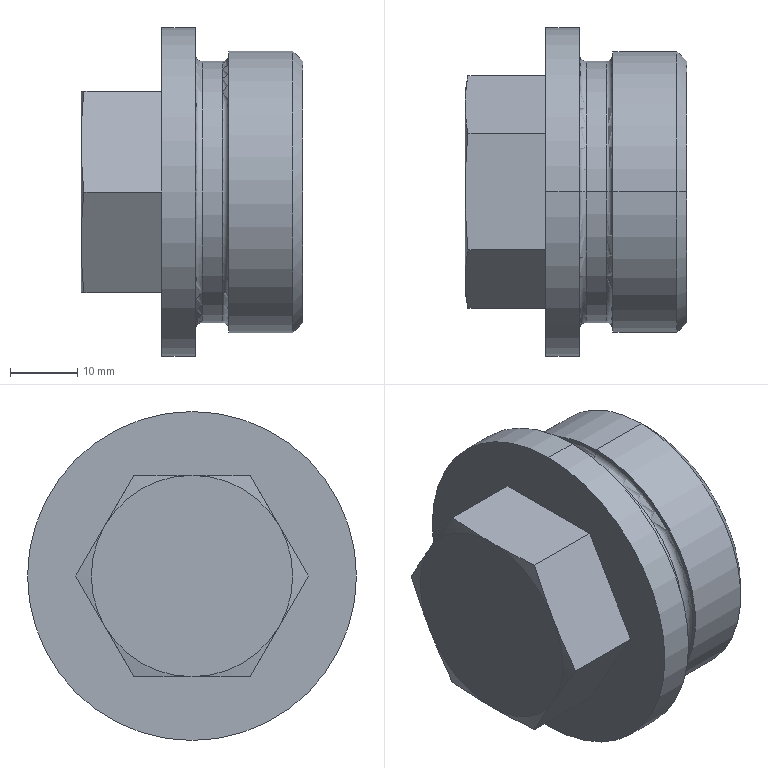Part | SolidWorks | features Boss 1, Cut 1, Fillet 1, Revolution 1 | 1 solid | 29 faces | box 33 x 49 x 49 mm | volume 39818 mm3 | plane 11 | cone 8 | cylinder 6 | torus 4 | commonest cylinder face diameters 38.952 x2 41.91 x2 49 x2
STEP:
#1=CARTESIAN_POINT('',(17.,0.,-20.476));
#2=VERTEX_POINT('',#1);
#3=CARTESIAN_POINT('',(17.,0.,20.476));
#4=VERTEX_POINT('',#3);
#5=CARTESIAN_POINT('',(17.,0.,0.));
#6=DIRECTION('',(-1.,0.,0.));
#7=DIRECTION('',(0.,0.,1.));
#8=AXIS2_PLACEMENT_3D('',#5,#6,#7);
#9=CIRCLE('',#8,20.476);
#10=EDGE_CURVE('',#2,#4,#9,.T.);
#11=ORIENTED_EDGE('',*,*,#10,.F.);
#12=CARTESIAN_POINT('',(18.,0.,-19.476));
#13=VERTEX_POINT('',#12);
#14=CARTESIAN_POINT('',(18.,0.,-20.476));
#15=DIRECTION('',(0.,1.,0.));
#16=DIRECTION('',(0.,0.,1.));
#17=AXIS2_PLACEMENT_3D('',#14,#15,#16);
#18=CIRCLE('',#17,1.);
#19=EDGE_CURVE('',#2,#13,#18,.T.);
#20=ORIENTED_EDGE('',*,*,#19,.T.);
#21=CARTESIAN_POINT('',(18.,0.,19.476));
#22=VERTEX_POINT('',#21);
#23=CARTESIAN_POINT('',(18.,0.,0.));
#24=DIRECTION('',(1.,0.,0.));
#25=DIRECTION('',(0.,0.,1.));
#26=AXIS2_PLACEMENT_3D('',#23,#24,#25);
#27=CIRCLE('',#26,19.476);
#28=EDGE_CURVE('',#22,#13,#27,.T.);
#29=ORIENTED_EDGE('',*,*,#28,.F.);
#30=CARTESIAN_POINT('',(18.,0.,20.476));
#31=DIRECTION('',(0.,-1.,0.));
#32=DIRECTION('',(0.,0.,-1.));
#33=AXIS2_PLACEMENT_3D('',#30,#31,#32);
#34=CIRCLE('',#33,1.);
#35=EDGE_CURVE('',#4,#22,#34,.T.);
#36=ORIENTED_EDGE('',*,*,#35,.F.);
#37=EDGE_LOOP('',(#11,#20,#29,#36));
#38=FACE_OUTER_BOUND('',#37,.T.);
#39=CARTESIAN_POINT('',(18.,0.,0.));
#40=DIRECTION('',(-1.,0.,0.));
#41=DIRECTION('',(0.,0.,1.));
#42=AXIS2_PLACEMENT_3D('',#39,#40,#41);
#43=TOROIDAL_SURFACE('',#42,20.476,1.);
#44=ADVANCED_FACE('',(#38),#43,.F.);
#45=CARTESIAN_POINT('',(22.,0.,20.476));
#46=VERTEX_POINT('',#45);
#47=CARTESIAN_POINT('',(22.,0.,-20.476));
#48=VERTEX_POINT('',#47);
#49=CARTESIAN_POINT('',(22.,0.,0.));
#50=DIRECTION('',(1.,0.,0.));
#51=DIRECTION('',(0.,0.,-1.));
#52=AXIS2_PLACEMENT_3D('',#49,#50,#51);
#53=CIRCLE('',#52,20.476);
#54=EDGE_CURVE('',#46,#48,#53,.T.);
#55=ORIENTED_EDGE('',*,*,#54,.F.);
#56=CARTESIAN_POINT('',(21.,0.,19.476));
#57=VERTEX_POINT('',#56);
#58=CARTESIAN_POINT('',(21.,0.,20.476));
#59=DIRECTION('',(0.,1.,0.));
#60=DIRECTION('',(0.,0.,1.));
#61=AXIS2_PLACEMENT_3D('',#58,#59,#60);
#62=CIRCLE('',#61,1.);
#63=EDGE_CURVE('',#46,#57,#62,.T.);
#64=ORIENTED_EDGE('',*,*,#63,.T.);
#65=CARTESIAN_POINT('',(21.,0.,-19.476));
#66=VERTEX_POINT('',#65);
#67=CARTESIAN_POINT('',(21.,0.,0.));
#68=DIRECTION('',(-1.,0.,0.));
#69=DIRECTION('',(0.,0.,-1.));
#70=AXIS2_PLACEMENT_3D('',#67,#68,#69);
#71=CIRCLE('',#70,19.476);
#72=EDGE_CURVE('',#66,#57,#71,.T.);
#73=ORIENTED_EDGE('',*,*,#72,.F.);
#74=CARTESIAN_POINT('',(21.,0.,-20.476));
#75=DIRECTION('',(0.,-1.,0.));
#76=DIRECTION('',(0.,0.,-1.));
#77=AXIS2_PLACEMENT_3D('',#74,#75,#76);
#78=CIRCLE('',#77,1.);
#79=EDGE_CURVE('',#48,#66,#78,.T.);
#80=ORIENTED_EDGE('',*,*,#79,.F.);
#81=EDGE_LOOP('',(#55,#64,#73,#80));
#82=FACE_OUTER_BOUND('',#81,.T.);
#83=CARTESIAN_POINT('',(21.,0.,0.));
#84=DIRECTION('',(1.,0.,0.));
#85=DIRECTION('',(0.,0.,-1.));
#86=AXIS2_PLACEMENT_3D('',#83,#84,#85);
#87=TOROIDAL_SURFACE('',#86,20.476,1.);
#88=ADVANCED_FACE('',(#82),#87,.F.);
#89=CARTESIAN_POINT('',(33.,0.,19.476));
#90=VERTEX_POINT('',#89);
#91=CARTESIAN_POINT('',(33.,0.,-19.476));
#92=VERTEX_POINT('',#91);
#93=CARTESIAN_POINT('',(33.,0.,0.));
#94=DIRECTION('',(-1.,0.,0.));
#95=DIRECTION('',(0.,0.,1.));
#96=AXIS2_PLACEMENT_3D('',#93,#94,#95);
#97=CIRCLE('',#96,19.476);
#98=EDGE_CURVE('',#90,#92,#97,.T.);
#99=ORIENTED_EDGE('',*,*,#98,.T.);
#100=CARTESIAN_POINT('',(31.521,0.,-20.955));
#101=VERTEX_POINT('',#100);
#102=CARTESIAN_POINT('',(33.,0.,-19.476));
#103=DIRECTION('',(-0.7071,0.,-0.7071));
#104=VECTOR('',#103,1000.);
#105=LINE('',#102,#104);
#106=EDGE_CURVE('',#92,#101,#105,.T.);
#107=ORIENTED_EDGE('',*,*,#106,.T.);
#108=CARTESIAN_POINT('',(31.521,0.,20.955));
#109=VERTEX_POINT('',#108);
#110=CARTESIAN_POINT('',(31.521,0.,0.));
#111=DIRECTION('',(-1.,0.,0.));
#112=DIRECTION('',(0.,0.,1.));
#113=AXIS2_PLACEMENT_3D('',#110,#111,#112);
#114=CIRCLE('',#113,20.955);
#115=EDGE_CURVE('',#109,#101,#114,.T.);
#116=ORIENTED_EDGE('',*,*,#115,.F.);
#117=CARTESIAN_POINT('',(33.,0.,19.476));
#118=DIRECTION('',(-0.7071,0.,0.7071));
#119=VECTOR('',#118,1000.);
#120=LINE('',#117,#119);
#121=EDGE_CURVE('',#90,#109,#120,.T.);
#122=ORIENTED_EDGE('',*,*,#121,.F.);
#123=EDGE_LOOP('',(#99,#107,#116,#122));
#124=FACE_OUTER_BOUND('',#123,.T.);
#125=CARTESIAN_POINT('',(33.,0.,0.));
#126=DIRECTION('',(-1.,0.,0.));
#127=DIRECTION('',(0.,0.,1.));
#128=AXIS2_PLACEMENT_3D('',#125,#126,#127);
#129=CONICAL_SURFACE('',#128,19.476,0.7854);
#130=ADVANCED_FACE('',(#124),#129,.T.);
#131=ORIENTED_EDGE('',*,*,#115,.T.);
#132=CARTESIAN_POINT('',(22.,0.,-20.955));
#133=VERTEX_POINT('',#132);
#134=CARTESIAN_POINT('',(0.,0.,-20.955));
#135=DIRECTION('',(-1.,0.,0.));
#136=VECTOR('',#135,1000.);
#137=LINE('',#134,#136);
#138=EDGE_CURVE('',#101,#133,#137,.T.);
#139=ORIENTED_EDGE('',*,*,#138,.T.);
#140=CARTESIAN_POINT('',(22.,0.,20.955));
#141=VERTEX_POINT('',#140);
#142=CARTESIAN_POINT('',(22.,0.,0.));
#143=DIRECTION('',(-1.,0.,0.));
#144=DIRECTION('',(0.,0.,1.));
#145=AXIS2_PLACEMENT_3D('',#142,#143,#144);
#146=CIRCLE('',#145,20.955);
#147=EDGE_CURVE('',#141,#133,#146,.T.);
#148=ORIENTED_EDGE('',*,*,#147,.F.);
#149=CARTESIAN_POINT('',(0.,0.,20.955));
#150=DIRECTION('',(-1.,0.,0.));
#151=VECTOR('',#150,1000.);
#152=LINE('',#149,#151);
#153=EDGE_CURVE('',#109,#141,#152,.T.);
#154=ORIENTED_EDGE('',*,*,#153,.F.);
#155=EDGE_LOOP('',(#131,#139,#148,#154));
#156=FACE_OUTER_BOUND('',#155,.T.);
#157=CARTESIAN_POINT('',(0.,0.,0.));
#158=DIRECTION('',(-1.,0.,0.));
#159=DIRECTION('',(0.,0.,1.));
#160=AXIS2_PLACEMENT_3D('',#157,#158,#159);
#161=CYLINDRICAL_SURFACE('',#160,20.955);
#162=ADVANCED_FACE('',(#156),#161,.T.);
#163=CARTESIAN_POINT('',(21.,0.,0.));
#164=DIRECTION('',(-1.,0.,0.));
#165=DIRECTION('',(0.,0.,-1.));
#166=AXIS2_PLACEMENT_3D('',#163,#164,#165);
#167=CIRCLE('',#166,19.476);
#168=EDGE_CURVE('',#57,#66,#167,.T.);
#169=ORIENTED_EDGE('',*,*,#168,.T.);
#170=CARTESIAN_POINT('',(0.,0.,-19.476));
#171=DIRECTION('',(-1.,0.,0.));
#172=VECTOR('',#171,1000.);
#173=LINE('',#170,#172);
#174=EDGE_CURVE('',#66,#13,#173,.T.);
#175=ORIENTED_EDGE('',*,*,#174,.T.);
#176=CARTESIAN_POINT('',(18.,0.,0.));
#177=DIRECTION('',(1.,0.,0.));
#178=DIRECTION('',(0.,0.,1.));
#179=AXIS2_PLACEMENT_3D('',#176,#177,#178);
#180=CIRCLE('',#179,19.476);
#181=EDGE_CURVE('',#13,#22,#180,.T.);
#182=ORIENTED_EDGE('',*,*,#181,.T.);
#183=CARTESIAN_POINT('',(0.,0.,19.476));
#184=DIRECTION('',(-1.,0.,0.));
#185=VECTOR('',#184,1000.);
#186=LINE('',#183,#185);
#187=EDGE_CURVE('',#57,#22,#186,.T.);
#188=ORIENTED_EDGE('',*,*,#187,.F.);
#189=EDGE_LOOP('',(#169,#175,#182,#188));
#190=FACE_OUTER_BOUND('',#189,.T.);
#191=CARTESIAN_POINT('',(0.,0.,0.));
#192=DIRECTION('',(-1.,0.,0.));
#193=DIRECTION('',(0.,0.,1.));
#194=AXIS2_PLACEMENT_3D('',#191,#192,#193);
#195=CYLINDRICAL_SURFACE('',#194,19.476);
#196=ADVANCED_FACE('',(#190),#195,.T.);
#197=CARTESIAN_POINT('',(17.,0.,24.5));
#198=VERTEX_POINT('',#197);
#199=CARTESIAN_POINT('',(17.,0.,-24.5));
#200=VERTEX_POINT('',#199);
#201=CARTESIAN_POINT('',(17.,0.,0.));
#202=DIRECTION('',(-1.,0.,0.));
#203=DIRECTION('',(0.,0.,1.));
#204=AXIS2_PLACEMENT_3D('',#201,#202,#203);
#205=CIRCLE('',#204,24.5);
#206=EDGE_CURVE('',#198,#200,#205,.T.);
#207=ORIENTED_EDGE('',*,*,#206,.T.);
#208=CARTESIAN_POINT('',(12.,0.,-24.5));
#209=VERTEX_POINT('',#208);
#210=CARTESIAN_POINT('',(0.,0.,-24.5));
#211=DIRECTION('',(-1.,0.,0.));
#212=VECTOR('',#211,1000.);
#213=LINE('',#210,#212);
#214=EDGE_CURVE('',#200,#209,#213,.T.);
#215=ORIENTED_EDGE('',*,*,#214,.T.);
#216=CARTESIAN_POINT('',(12.,0.,24.5));
#217=VERTEX_POINT('',#216);
#218=CARTESIAN_POINT('',(12.,0.,0.));
#219=DIRECTION('',(-1.,0.,0.));
#220=DIRECTION('',(0.,0.,1.));
#221=AXIS2_PLACEMENT_3D('',#218,#219,#220);
#222=CIRCLE('',#221,24.5);
#223=EDGE_CURVE('',#217,#209,#222,.T.);
#224=ORIENTED_EDGE('',*,*,#223,.F.);
#225=CARTESIAN_POINT('',(0.,0.,24.5));
#226=DIRECTION('',(-1.,0.,0.));
#227=VECTOR('',#226,1000.);
#228=LINE('',#225,#227);
#229=EDGE_CURVE('',#198,#217,#228,.T.);
#230=ORIENTED_EDGE('',*,*,#229,.F.);
#231=EDGE_LOOP('',(#207,#215,#224,#230));
#232=FACE_OUTER_BOUND('',#231,.T.);
#233=CARTESIAN_POINT('',(0.,0.,0.));
#234=DIRECTION('',(-1.,0.,0.));
#235=DIRECTION('',(0.,0.,1.));
#236=AXIS2_PLACEMENT_3D('',#233,#234,#235);
#237=CYLINDRICAL_SURFACE('',#236,24.5);
#238=ADVANCED_FACE('',(#232),#237,.T.);
#239=CARTESIAN_POINT('',(12.,8.66,-15.));
#240=VERTEX_POINT('',#239);
#241=CARTESIAN_POINT('',(0.4092,8.66,-15.));
#242=VERTEX_POINT('',#241);
#243=CARTESIAN_POINT('',(57.826,8.66,-15.));
#244=DIRECTION('',(-1.,0.,0.));
#245=VECTOR('',#244,1000.);
#246=LINE('',#243,#245);
#247=EDGE_CURVE('',#240,#242,#246,.T.);
#248=ORIENTED_EDGE('',*,*,#247,.T.);
#249=CARTESIAN_POINT('',(0.,12.99,-7.5));
#250=VERTEX_POINT('',#249);
#251=CARTESIAN_POINT('',(0.4092,8.66,-15.));
#252=CARTESIAN_POINT('',(0.2819,9.382,-13.75));
#253=CARTESIAN_POINT('',(0.1786,10.104,-12.5));
#254=CARTESIAN_POINT('',(0.03741,11.547,-10.));
#255=CARTESIAN_POINT('',(0.,12.269,-8.75));
#256=CARTESIAN_POINT('',(0.,12.99,-7.5));
#257=B_SPLINE_CURVE_WITH_KNOTS('',3,(#251,#252,#253,#254,#255,#256),.UNSPECIFIED.,.F.,.F.,(4,2,4),(0.000000231,0.00433,0.00866),.UNSPECIFIED.);
#258=EDGE_CURVE('',#242,#250,#257,.T.);
#259=ORIENTED_EDGE('',*,*,#258,.T.);
#260=CARTESIAN_POINT('',(0.4092,17.321,0.));
#261=VERTEX_POINT('',#260);
#262=CARTESIAN_POINT('',(0.,12.99,-7.5));
#263=CARTESIAN_POINT('',(0.,13.712,-6.25));
#264=CARTESIAN_POINT('',(0.03741,14.434,-5.));
#265=CARTESIAN_POINT('',(0.1786,15.877,-2.5));
#266=CARTESIAN_POINT('',(0.2819,16.599,-1.25));
#267=CARTESIAN_POINT('',(0.4092,17.321,0.));
#268=B_SPLINE_CURVE_WITH_KNOTS('',3,(#262,#263,#264,#265,#266,#267),.UNSPECIFIED.,.F.,.F.,(4,2,4),(0.00866,0.01299,0.01732),.UNSPECIFIED.);
#269=EDGE_CURVE('',#250,#261,#268,.T.);
#270=ORIENTED_EDGE('',*,*,#269,.T.);
#271=CARTESIAN_POINT('',(12.,17.321,0.));
#272=VERTEX_POINT('',#271);
#273=CARTESIAN_POINT('',(57.826,17.321,0.));
#274=DIRECTION('',(-1.,0.,0.));
#275=VECTOR('',#274,1000.);
#276=LINE('',#273,#275);
#277=EDGE_CURVE('',#272,#261,#276,.T.);
#278=ORIENTED_EDGE('',*,*,#277,.F.);
#279=CARTESIAN_POINT('',(12.,17.321,0.));
#280=DIRECTION('',(0.,-0.5,-0.866));
#281=VECTOR('',#280,1000.);
#282=LINE('',#279,#281);
#283=EDGE_CURVE('',#272,#240,#282,.T.);
#284=ORIENTED_EDGE('',*,*,#283,.T.);
#285=EDGE_LOOP('',(#248,#259,#270,#278,#284));
#286=FACE_OUTER_BOUND('',#285,.T.);
#287=CARTESIAN_POINT('',(57.826,17.321,0.));
#288=DIRECTION('',(0.,0.866,-0.5));
#289=DIRECTION('',(0.,0.5,0.866));
#290=AXIS2_PLACEMENT_3D('',#287,#288,#289);
#291=PLANE('',#290);
#292=ADVANCED_FACE('',(#286),#291,.T.);
#293=CARTESIAN_POINT('',(12.,-8.66,-15.));
#294=VERTEX_POINT('',#293);
#295=CARTESIAN_POINT('',(0.4092,-8.66,-15.));
#296=VERTEX_POINT('',#295);
#297=CARTESIAN_POINT('',(57.826,-8.66,-15.));
#298=DIRECTION('',(-1.,0.,0.));
#299=VECTOR('',#298,1000.);
#300=LINE('',#297,#299);
#301=EDGE_CURVE('',#294,#296,#300,.T.);
#302=ORIENTED_EDGE('',*,*,#301,.T.);
#303=CARTESIAN_POINT('',(0.,0.,-15.));
#304=VERTEX_POINT('',#303);
#305=CARTESIAN_POINT('',(0.4092,-8.66,-15.));
#306=CARTESIAN_POINT('',(0.2821,-7.219,-15.));
#307=CARTESIAN_POINT('',(0.1786,-5.773,-15.));
#308=CARTESIAN_POINT('',(0.03738,-2.886,-15.));
#309=CARTESIAN_POINT('',(0.,-1.443,-15.));
#310=CARTESIAN_POINT('',(0.,0.,-15.));
#311=B_SPLINE_CURVE_WITH_KNOTS('',3,(#305,#306,#307,#308,#309,#310),.UNSPECIFIED.,.F.,.F.,(4,2,4),(0.01454,0.01888,0.02322),.UNSPECIFIED.);
#312=EDGE_CURVE('',#296,#304,#311,.T.);
#313=ORIENTED_EDGE('',*,*,#312,.T.);
#314=CARTESIAN_POINT('',(0.,0.,-15.));
#315=CARTESIAN_POINT('',(0.,1.445,-15.));
#316=CARTESIAN_POINT('',(0.03747,2.888,-15.));
#317=CARTESIAN_POINT('',(0.1787,5.775,-15.));
#318=CARTESIAN_POINT('',(0.282,7.218,-15.));
#319=CARTESIAN_POINT('',(0.4092,8.66,-15.));
#320=B_SPLINE_CURVE_WITH_KNOTS('',3,(#314,#315,#316,#317,#318,#319),.UNSPECIFIED.,.F.,.F.,(4,2,4),(0.02322,0.02756,0.03191),.UNSPECIFIED.);
#321=EDGE_CURVE('',#304,#242,#320,.T.);
#322=ORIENTED_EDGE('',*,*,#321,.T.);
#323=ORIENTED_EDGE('',*,*,#247,.F.);
#324=CARTESIAN_POINT('',(12.,8.66,-15.));
#325=DIRECTION('',(0.,-1.,0.));
#326=VECTOR('',#325,1000.);
#327=LINE('',#324,#326);
#328=EDGE_CURVE('',#240,#294,#327,.T.);
#329=ORIENTED_EDGE('',*,*,#328,.T.);
#330=EDGE_LOOP('',(#302,#313,#322,#323,#329));
#331=FACE_OUTER_BOUND('',#330,.T.);
#332=CARTESIAN_POINT('',(57.826,8.66,-15.));
#333=DIRECTION('',(0.,0.,-1.));
#334=DIRECTION('',(0.,1.,0.));
#335=AXIS2_PLACEMENT_3D('',#332,#333,#334);
#336=PLANE('',#335);
#337=ADVANCED_FACE('',(#331),#336,.T.);
#338=CARTESIAN_POINT('',(12.,-17.321,0.));
#339=VERTEX_POINT('',#338);
#340=CARTESIAN_POINT('',(0.4092,-17.321,0.));
#341=VERTEX_POINT('',#340);
#342=CARTESIAN_POINT('',(57.826,-17.321,0.));
#343=DIRECTION('',(-1.,0.,0.));
#344=VECTOR('',#343,1000.);
#345=LINE('',#342,#344);
#346=EDGE_CURVE('',#339,#341,#345,.T.);
#347=ORIENTED_EDGE('',*,*,#346,.T.);
#348=CARTESIAN_POINT('',(0.,-12.99,-7.5));
#349=VERTEX_POINT('',#348);
#350=CARTESIAN_POINT('',(0.4092,-17.321,0.));
#351=CARTESIAN_POINT('',(0.2819,-16.599,-1.25));
#352=CARTESIAN_POINT('',(0.1786,-15.877,-2.5));
#353=CARTESIAN_POINT('',(0.03741,-14.434,-5.));
#354=CARTESIAN_POINT('',(0.,-13.712,-6.25));
#355=CARTESIAN_POINT('',(0.,-12.99,-7.5));
#356=B_SPLINE_CURVE_WITH_KNOTS('',3,(#350,#351,#352,#353,#354,#355),.UNSPECIFIED.,.F.,.F.,(4,2,4),(0.000000231,0.00433,0.00866),.UNSPECIFIED.);
#357=EDGE_CURVE('',#341,#349,#356,.T.);
#358=ORIENTED_EDGE('',*,*,#357,.T.);
#359=CARTESIAN_POINT('',(0.,-12.99,-7.5));
#360=CARTESIAN_POINT('',(0.,-12.269,-8.75));
#361=CARTESIAN_POINT('',(0.03741,-11.547,-10.));
#362=CARTESIAN_POINT('',(0.1786,-10.104,-12.5));
#363=CARTESIAN_POINT('',(0.2819,-9.382,-13.75));
#364=CARTESIAN_POINT('',(0.4092,-8.66,-15.));
#365=B_SPLINE_CURVE_WITH_KNOTS('',3,(#359,#360,#361,#362,#363,#364),.UNSPECIFIED.,.F.,.F.,(4,2,4),(0.00866,0.01299,0.01732),.UNSPECIFIED.);
#366=EDGE_CURVE('',#349,#296,#365,.T.);
#367=ORIENTED_EDGE('',*,*,#366,.T.);
#368=ORIENTED_EDGE('',*,*,#301,.F.);
#369=CARTESIAN_POINT('',(12.,-8.66,-15.));
#370=DIRECTION('',(0.,-0.5,0.866));
#371=VECTOR('',#370,1000.);
#372=LINE('',#369,#371);
#373=EDGE_CURVE('',#294,#339,#372,.T.);
#374=ORIENTED_EDGE('',*,*,#373,.T.);
#375=EDGE_LOOP('',(#347,#358,#367,#368,#374));
#376=FACE_OUTER_BOUND('',#375,.T.);
#377=CARTESIAN_POINT('',(57.826,-8.66,-15.));
#378=DIRECTION('',(0.,-0.866,-0.5));
#379=DIRECTION('',(0.,0.5,-0.866));
#380=AXIS2_PLACEMENT_3D('',#377,#378,#379);
#381=PLANE('',#380);
#382=ADVANCED_FACE('',(#376),#381,.T.);
#383=CARTESIAN_POINT('',(12.,-8.66,15.));
#384=VERTEX_POINT('',#383);
#385=CARTESIAN_POINT('',(0.4092,-8.66,15.));
#386=VERTEX_POINT('',#385);
#387=CARTESIAN_POINT('',(57.826,-8.66,15.));
#388=DIRECTION('',(-1.,0.,0.));
#389=VECTOR('',#388,1000.);
#390=LINE('',#387,#389);
#391=EDGE_CURVE('',#384,#386,#390,.T.);
#392=ORIENTED_EDGE('',*,*,#391,.T.);
#393=CARTESIAN_POINT('',(0.,-12.99,7.5));
#394=VERTEX_POINT('',#393);
#395=CARTESIAN_POINT('',(0.4092,-8.66,15.));
#396=CARTESIAN_POINT('',(0.2819,-9.382,13.75));
#397=CARTESIAN_POINT('',(0.1786,-10.104,12.5));
#398=CARTESIAN_POINT('',(0.03741,-11.547,10.));
#399=CARTESIAN_POINT('',(0.,-12.269,8.75));
#400=CARTESIAN_POINT('',(0.,-12.99,7.5));
#401=B_SPLINE_CURVE_WITH_KNOTS('',3,(#395,#396,#397,#398,#399,#400),.UNSPECIFIED.,.F.,.F.,(4,2,4),(0.000000231,0.00433,0.00866),.UNSPECIFIED.);
#402=EDGE_CURVE('',#386,#394,#401,.T.);
#403=ORIENTED_EDGE('',*,*,#402,.T.);
#404=CARTESIAN_POINT('',(0.,-12.99,7.5));
#405=CARTESIAN_POINT('',(0.,-13.712,6.25));
#406=CARTESIAN_POINT('',(0.03741,-14.434,5.));
#407=CARTESIAN_POINT('',(0.1786,-15.877,2.5));
#408=CARTESIAN_POINT('',(0.2819,-16.599,1.25));
#409=CARTESIAN_POINT('',(0.4092,-17.321,0.));
#410=B_SPLINE_CURVE_WITH_KNOTS('',3,(#404,#405,#406,#407,#408,#409),.UNSPECIFIED.,.F.,.F.,(4,2,4),(0.00866,0.01299,0.01732),.UNSPECIFIED.);
#411=EDGE_CURVE('',#394,#341,#410,.T.);
#412=ORIENTED_EDGE('',*,*,#411,.T.);
#413=ORIENTED_EDGE('',*,*,#346,.F.);
#414=CARTESIAN_POINT('',(12.,-17.321,0.));
#415=DIRECTION('',(0.,0.5,0.866));
#416=VECTOR('',#415,1000.);
#417=LINE('',#414,#416);
#418=EDGE_CURVE('',#339,#384,#417,.T.);
#419=ORIENTED_EDGE('',*,*,#418,.T.);
#420=EDGE_LOOP('',(#392,#403,#412,#413,#419));
#421=FACE_OUTER_BOUND('',#420,.T.);
#422=CARTESIAN_POINT('',(57.826,-17.321,0.));
#423=DIRECTION('',(0.,-0.866,0.5));
#424=DIRECTION('',(0.,-0.5,-0.866));
#425=AXIS2_PLACEMENT_3D('',#422,#423,#424);
#426=PLANE('',#425);
#427=ADVANCED_FACE('',(#421),#426,.T.);
#428=CARTESIAN_POINT('',(12.,8.66,15.));
#429=VERTEX_POINT('',#428);
#430=CARTESIAN_POINT('',(0.4092,8.66,15.));
#431=VERTEX_POINT('',#430);
#432=CARTESIAN_POINT('',(57.826,8.66,15.));
#433=DIRECTION('',(-1.,0.,0.));
#434=VECTOR('',#433,1000.);
#435=LINE('',#432,#434);
#436=EDGE_CURVE('',#429,#431,#435,.T.);
#437=ORIENTED_EDGE('',*,*,#436,.T.);
#438=CARTESIAN_POINT('',(0.,0.,15.));
#439=VERTEX_POINT('',#438);
#440=CARTESIAN_POINT('',(0.4092,8.66,15.));
#441=CARTESIAN_POINT('',(0.282,7.218,15.));
#442=CARTESIAN_POINT('',(0.1787,5.775,15.));
#443=CARTESIAN_POINT('',(0.03747,2.888,15.));
#444=CARTESIAN_POINT('',(0.,1.445,15.));
#445=CARTESIAN_POINT('',(0.,0.,15.));
#446=B_SPLINE_CURVE_WITH_KNOTS('',3,(#440,#441,#442,#443,#444,#445),.UNSPECIFIED.,.F.,.F.,(4,2,4),(0.0406,0.04494,0.04928),.UNSPECIFIED.);
#447=EDGE_CURVE('',#431,#439,#446,.T.);
#448=ORIENTED_EDGE('',*,*,#447,.T.);
#449=CARTESIAN_POINT('',(0.,0.,15.));
#450=CARTESIAN_POINT('',(0.,-1.443,15.));
#451=CARTESIAN_POINT('',(0.03738,-2.886,15.));
#452=CARTESIAN_POINT('',(0.1786,-5.773,15.));
#453=CARTESIAN_POINT('',(0.2821,-7.219,15.));
#454=CARTESIAN_POINT('',(0.4092,-8.66,15.));
#455=B_SPLINE_CURVE_WITH_KNOTS('',3,(#449,#450,#451,#452,#453,#454),.UNSPECIFIED.,.F.,.F.,(4,2,4),(0.04928,0.05362,0.05795),.UNSPECIFIED.);
#456=EDGE_CURVE('',#439,#386,#455,.T.);
#457=ORIENTED_EDGE('',*,*,#456,.T.);
#458=ORIENTED_EDGE('',*,*,#391,.F.);
#459=CARTESIAN_POINT('',(12.,-8.66,15.));
#460=DIRECTION('',(0.,1.,0.));
#461=VECTOR('',#460,1000.);
#462=LINE('',#459,#461);
#463=EDGE_CURVE('',#384,#429,#462,.T.);
#464=ORIENTED_EDGE('',*,*,#463,.T.);
#465=EDGE_LOOP('',(#437,#448,#457,#458,#464));
#466=FACE_OUTER_BOUND('',#465,.T.);
#467=CARTESIAN_POINT('',(57.826,-8.66,15.));
#468=DIRECTION('',(0.,0.,1.));
#469=DIRECTION('',(0.,-1.,0.));
#470=AXIS2_PLACEMENT_3D('',#467,#468,#469);
#471=PLANE('',#470);
#472=ADVANCED_FACE('',(#466),#471,.T.);
#473=ORIENTED_EDGE('',*,*,#277,.T.);
#474=CARTESIAN_POINT('',(0.,12.99,7.5));
#475=VERTEX_POINT('',#474);
#476=CARTESIAN_POINT('',(0.4092,17.321,0.));
#477=CARTESIAN_POINT('',(0.2819,16.599,1.25));
#478=CARTESIAN_POINT('',(0.1786,15.877,2.5));
#479=CARTESIAN_POINT('',(0.03741,14.434,5.));
#480=CARTESIAN_POINT('',(0.,13.712,6.25));
#481=CARTESIAN_POINT('',(0.,12.99,7.5));
#482=B_SPLINE_CURVE_WITH_KNOTS('',3,(#476,#477,#478,#479,#480,#481),.UNSPECIFIED.,.F.,.F.,(4,2,4),(0.000000231,0.00433,0.00866),.UNSPECIFIED.);
#483=EDGE_CURVE('',#261,#475,#482,.T.);
#484=ORIENTED_EDGE('',*,*,#483,.T.);
#485=CARTESIAN_POINT('',(0.,12.99,7.5));
#486=CARTESIAN_POINT('',(0.,12.269,8.75));
#487=CARTESIAN_POINT('',(0.03741,11.547,10.));
#488=CARTESIAN_POINT('',(0.1786,10.104,12.5));
#489=CARTESIAN_POINT('',(0.2819,9.382,13.75));
#490=CARTESIAN_POINT('',(0.4092,8.66,15.));
#491=B_SPLINE_CURVE_WITH_KNOTS('',3,(#485,#486,#487,#488,#489,#490),.UNSPECIFIED.,.F.,.F.,(4,2,4),(0.00866,0.01299,0.01732),.UNSPECIFIED.);
#492=EDGE_CURVE('',#475,#431,#491,.T.);
#493=ORIENTED_EDGE('',*,*,#492,.T.);
#494=ORIENTED_EDGE('',*,*,#436,.F.);
#495=CARTESIAN_POINT('',(12.,8.66,15.));
#496=DIRECTION('',(0.,0.5,-0.866));
#497=VECTOR('',#496,1000.);
#498=LINE('',#495,#497);
#499=EDGE_CURVE('',#429,#272,#498,.T.);
#500=ORIENTED_EDGE('',*,*,#499,.T.);
#501=EDGE_LOOP('',(#473,#484,#493,#494,#500));
#502=FACE_OUTER_BOUND('',#501,.T.);
#503=CARTESIAN_POINT('',(57.826,8.66,15.));
#504=DIRECTION('',(0.,0.866,0.5));
#505=DIRECTION('',(0.,-0.5,0.866));
#506=AXIS2_PLACEMENT_3D('',#503,#504,#505);
#507=PLANE('',#506);
#508=ADVANCED_FACE('',(#502),#507,.T.);
#509=ORIENTED_EDGE('',*,*,#328,.F.);
#510=ORIENTED_EDGE('',*,*,#283,.F.);
#511=ORIENTED_EDGE('',*,*,#499,.F.);
#512=ORIENTED_EDGE('',*,*,#463,.F.);
#513=ORIENTED_EDGE('',*,*,#418,.F.);
#514=ORIENTED_EDGE('',*,*,#373,.F.);
#515=EDGE_LOOP('',(#509,#510,#511,#512,#513,#514));
#516=FACE_BOUND('',#515,.T.);
#517=ORIENTED_EDGE('',*,*,#223,.T.);
#518=CARTESIAN_POINT('',(12.,0.,0.));
#519=DIRECTION('',(-1.,0.,0.));
#520=DIRECTION('',(0.,0.,1.));
#521=AXIS2_PLACEMENT_3D('',#518,#519,#520);
#522=CIRCLE('',#521,24.5);
#523=EDGE_CURVE('',#209,#217,#522,.T.);
#524=ORIENTED_EDGE('',*,*,#523,.T.);
#525=EDGE_LOOP('',(#517,#524));
#526=FACE_OUTER_BOUND('',#525,.T.);
#527=CARTESIAN_POINT('',(12.,24.5,0.));
#528=DIRECTION('',(1.,0.,0.));
#529=DIRECTION('',(0.,0.,-1.));
#530=AXIS2_PLACEMENT_3D('',#527,#528,#529);
#531=PLANE('',#530);
#532=ADVANCED_FACE('',(#516,#526),#531,.F.);
#533=ORIENTED_EDGE('',*,*,#214,.F.);
#534=CARTESIAN_POINT('',(17.,0.,0.));
#535=DIRECTION('',(-1.,0.,0.));
#536=DIRECTION('',(0.,0.,1.));
#537=AXIS2_PLACEMENT_3D('',#534,#535,#536);
#538=CIRCLE('',#537,24.5);
#539=EDGE_CURVE('',#200,#198,#538,.T.);
#540=ORIENTED_EDGE('',*,*,#539,.T.);
#541=ORIENTED_EDGE('',*,*,#229,.T.);
#542=ORIENTED_EDGE('',*,*,#523,.F.);
#543=EDGE_LOOP('',(#533,#540,#541,#542));
#544=FACE_OUTER_BOUND('',#543,.T.);
#545=CARTESIAN_POINT('',(0.,0.,0.));
#546=DIRECTION('',(-1.,0.,0.));
#547=DIRECTION('',(0.,0.,1.));
#548=AXIS2_PLACEMENT_3D('',#545,#546,#547);
#549=CYLINDRICAL_SURFACE('',#548,24.5);
#550=ADVANCED_FACE('',(#544),#549,.T.);
#551=CARTESIAN_POINT('',(17.,0.,0.));
#552=DIRECTION('',(-1.,0.,0.));
#553=DIRECTION('',(0.,0.,1.));
#554=AXIS2_PLACEMENT_3D('',#551,#552,#553);
#555=CIRCLE('',#554,20.476);
#556=EDGE_CURVE('',#4,#2,#555,.T.);
#557=ORIENTED_EDGE('',*,*,#556,.T.);
#558=ORIENTED_EDGE('',*,*,#10,.T.);
#559=EDGE_LOOP('',(#557,#558));
#560=FACE_BOUND('',#559,.T.);
#561=ORIENTED_EDGE('',*,*,#206,.F.);
#562=ORIENTED_EDGE('',*,*,#539,.F.);
#563=EDGE_LOOP('',(#561,#562));
#564=FACE_OUTER_BOUND('',#563,.T.);
#565=CARTESIAN_POINT('',(17.,19.476,0.));
#566=DIRECTION('',(-1.,0.,0.));
#567=DIRECTION('',(0.,0.,1.));
#568=AXIS2_PLACEMENT_3D('',#565,#566,#567);
#569=PLANE('',#568);
#570=ADVANCED_FACE('',(#560,#564),#569,.F.);
#571=ORIENTED_EDGE('',*,*,#174,.F.);
#572=ORIENTED_EDGE('',*,*,#72,.T.);
#573=ORIENTED_EDGE('',*,*,#187,.T.);
#574=ORIENTED_EDGE('',*,*,#28,.T.);
#575=EDGE_LOOP('',(#571,#572,#573,#574));
#576=FACE_OUTER_BOUND('',#575,.T.);
#577=CARTESIAN_POINT('',(0.,0.,0.));
#578=DIRECTION('',(-1.,0.,0.));
#579=DIRECTION('',(0.,0.,1.));
#580=AXIS2_PLACEMENT_3D('',#577,#578,#579);
#581=CYLINDRICAL_SURFACE('',#580,19.476);
#582=ADVANCED_FACE('',(#576),#581,.T.);
#583=CARTESIAN_POINT('',(22.,0.,0.));
#584=DIRECTION('',(1.,0.,0.));
#585=DIRECTION('',(0.,0.,-1.));
#586=AXIS2_PLACEMENT_3D('',#583,#584,#585);
#587=CIRCLE('',#586,20.476);
#588=EDGE_CURVE('',#48,#46,#587,.T.);
#589=ORIENTED_EDGE('',*,*,#588,.T.);
#590=ORIENTED_EDGE('',*,*,#54,.T.);
#591=EDGE_LOOP('',(#589,#590));
#592=FACE_BOUND('',#591,.T.);
#593=ORIENTED_EDGE('',*,*,#147,.T.);
#594=CARTESIAN_POINT('',(22.,0.,0.));
#595=DIRECTION('',(-1.,0.,0.));
#596=DIRECTION('',(0.,0.,1.));
#597=AXIS2_PLACEMENT_3D('',#594,#595,#596);
#598=CIRCLE('',#597,20.955);
#599=EDGE_CURVE('',#133,#141,#598,.T.);
#600=ORIENTED_EDGE('',*,*,#599,.T.);
#601=EDGE_LOOP('',(#593,#600));
#602=FACE_OUTER_BOUND('',#601,.T.);
#603=CARTESIAN_POINT('',(22.,20.955,0.));
#604=DIRECTION('',(1.,0.,0.));
#605=DIRECTION('',(0.,0.,-1.));
#606=AXIS2_PLACEMENT_3D('',#603,#604,#605);
#607=PLANE('',#606);
#608=ADVANCED_FACE('',(#592,#602),#607,.F.);
#609=ORIENTED_EDGE('',*,*,#138,.F.);
#610=CARTESIAN_POINT('',(31.521,0.,0.));
#611=DIRECTION('',(-1.,0.,0.));
#612=DIRECTION('',(0.,0.,1.));
#613=AXIS2_PLACEMENT_3D('',#610,#611,#612);
#614=CIRCLE('',#613,20.955);
#615=EDGE_CURVE('',#101,#109,#614,.T.);
#616=ORIENTED_EDGE('',*,*,#615,.T.);
#617=ORIENTED_EDGE('',*,*,#153,.T.);
#618=ORIENTED_EDGE('',*,*,#599,.F.);
#619=EDGE_LOOP('',(#609,#616,#617,#618));
#620=FACE_OUTER_BOUND('',#619,.T.);
#621=CARTESIAN_POINT('',(0.,0.,0.));
#622=DIRECTION('',(-1.,0.,0.));
#623=DIRECTION('',(0.,0.,1.));
#624=AXIS2_PLACEMENT_3D('',#621,#622,#623);
#625=CYLINDRICAL_SURFACE('',#624,20.955);
#626=ADVANCED_FACE('',(#620),#625,.T.);
#627=ORIENTED_EDGE('',*,*,#106,.F.);
#628=CARTESIAN_POINT('',(33.,0.,0.));
#629=DIRECTION('',(-1.,0.,0.));
#630=DIRECTION('',(0.,0.,1.));
#631=AXIS2_PLACEMENT_3D('',#628,#629,#630);
#632=CIRCLE('',#631,19.476);
#633=EDGE_CURVE('',#92,#90,#632,.T.);
#634=ORIENTED_EDGE('',*,*,#633,.T.);
#635=ORIENTED_EDGE('',*,*,#121,.T.);
#636=ORIENTED_EDGE('',*,*,#615,.F.);
#637=EDGE_LOOP('',(#627,#634,#635,#636));
#638=FACE_OUTER_BOUND('',#637,.T.);
#639=CARTESIAN_POINT('',(33.,0.,0.));
#640=DIRECTION('',(-1.,0.,0.));
#641=DIRECTION('',(0.,0.,1.));
#642=AXIS2_PLACEMENT_3D('',#639,#640,#641);
#643=CONICAL_SURFACE('',#642,19.476,0.7854);
#644=ADVANCED_FACE('',(#638),#643,.T.);
#645=ORIENTED_EDGE('',*,*,#98,.F.);
#646=ORIENTED_EDGE('',*,*,#633,.F.);
#647=EDGE_LOOP('',(#645,#646));
#648=FACE_OUTER_BOUND('',#647,.T.);
#649=CARTESIAN_POINT('',(33.,19.476,0.));
#650=DIRECTION('',(-1.,0.,0.));
#651=DIRECTION('',(0.,0.,1.));
#652=AXIS2_PLACEMENT_3D('',#649,#650,#651);
#653=PLANE('',#652);
#654=ADVANCED_FACE('',(#648),#653,.F.);
#655=CARTESIAN_POINT('',(0.,0.,0.));
#656=DIRECTION('',(1.,0.,0.));
#657=DIRECTION('',(0.,0.,-1.));
#658=AXIS2_PLACEMENT_3D('',#655,#656,#657);
#659=CIRCLE('',#658,15.);
#660=EDGE_CURVE('',#349,#304,#659,.T.);
#661=ORIENTED_EDGE('',*,*,#660,.T.);
#662=ORIENTED_EDGE('',*,*,#312,.F.);
#663=ORIENTED_EDGE('',*,*,#366,.F.);
#664=EDGE_LOOP('',(#661,#662,#663));
#665=FACE_OUTER_BOUND('',#664,.T.);
#666=CARTESIAN_POINT('',(0.,0.,0.));
#667=DIRECTION('',(1.,0.,0.));
#668=DIRECTION('',(0.,0.,1.));
#669=AXIS2_PLACEMENT_3D('',#666,#667,#668);
#670=CONICAL_SURFACE('',#669,15.,1.396);
#671=ADVANCED_FACE('',(#665),#670,.T.);
#672=ORIENTED_EDGE('',*,*,#411,.F.);
#673=CARTESIAN_POINT('',(0.,0.,0.));
#674=DIRECTION('',(1.,0.,0.));
#675=DIRECTION('',(0.,0.,-1.));
#676=AXIS2_PLACEMENT_3D('',#673,#674,#675);
#677=CIRCLE('',#676,15.);
#678=EDGE_CURVE('',#394,#349,#677,.T.);
#679=ORIENTED_EDGE('',*,*,#678,.T.);
#680=ORIENTED_EDGE('',*,*,#357,.F.);
#681=EDGE_LOOP('',(#672,#679,#680));
#682=FACE_OUTER_BOUND('',#681,.T.);
#683=CARTESIAN_POINT('',(0.,0.,0.));
#684=DIRECTION('',(1.,0.,0.));
#685=DIRECTION('',(0.,0.,1.));
#686=AXIS2_PLACEMENT_3D('',#683,#684,#685);
#687=CONICAL_SURFACE('',#686,15.,1.396);
#688=ADVANCED_FACE('',(#682),#687,.T.);
#689=ORIENTED_EDGE('',*,*,#456,.F.);
#690=CARTESIAN_POINT('',(0.,0.,0.));
#691=DIRECTION('',(1.,0.,0.));
#692=DIRECTION('',(0.,0.,-1.));
#693=AXIS2_PLACEMENT_3D('',#690,#691,#692);
#694=CIRCLE('',#693,15.);
#695=EDGE_CURVE('',#439,#394,#694,.T.);
#696=ORIENTED_EDGE('',*,*,#695,.T.);
#697=ORIENTED_EDGE('',*,*,#402,.F.);
#698=EDGE_LOOP('',(#689,#696,#697));
#699=FACE_OUTER_BOUND('',#698,.T.);
#700=CARTESIAN_POINT('',(0.,0.,0.));
#701=DIRECTION('',(1.,0.,0.));
#702=DIRECTION('',(0.,0.,1.));
#703=AXIS2_PLACEMENT_3D('',#700,#701,#702);
#704=CONICAL_SURFACE('',#703,15.,1.396);
#705=ADVANCED_FACE('',(#699),#704,.T.);
#706=ORIENTED_EDGE('',*,*,#492,.F.);
#707=CARTESIAN_POINT('',(0.,0.,0.));
#708=DIRECTION('',(-1.,0.,0.));
#709=DIRECTION('',(0.,0.,1.));
#710=AXIS2_PLACEMENT_3D('',#707,#708,#709);
#711=CIRCLE('',#710,15.);
#712=EDGE_CURVE('',#439,#475,#711,.T.);
#713=ORIENTED_EDGE('',*,*,#712,.F.);
#714=ORIENTED_EDGE('',*,*,#447,.F.);
#715=EDGE_LOOP('',(#706,#713,#714));
#716=FACE_OUTER_BOUND('',#715,.T.);
#717=CARTESIAN_POINT('',(0.,0.,0.));
#718=DIRECTION('',(1.,0.,0.));
#719=DIRECTION('',(0.,0.,1.));
#720=AXIS2_PLACEMENT_3D('',#717,#718,#719);
#721=CONICAL_SURFACE('',#720,15.,1.396);
#722=ADVANCED_FACE('',(#716),#721,.T.);
#723=CARTESIAN_POINT('',(0.,0.,0.));
#724=DIRECTION('',(1.,0.,0.));
#725=DIRECTION('',(0.,0.,-1.));
#726=AXIS2_PLACEMENT_3D('',#723,#724,#725);
#727=CIRCLE('',#726,15.);
#728=EDGE_CURVE('',#250,#475,#727,.T.);
#729=ORIENTED_EDGE('',*,*,#728,.T.);
#730=ORIENTED_EDGE('',*,*,#483,.F.);
#731=ORIENTED_EDGE('',*,*,#269,.F.);
#732=EDGE_LOOP('',(#729,#730,#731));
#733=FACE_OUTER_BOUND('',#732,.T.);
#734=CARTESIAN_POINT('',(0.,0.,0.));
#735=DIRECTION('',(1.,0.,0.));
#736=DIRECTION('',(0.,0.,1.));
#737=AXIS2_PLACEMENT_3D('',#734,#735,#736);
#738=CONICAL_SURFACE('',#737,15.,1.396);
#739=ADVANCED_FACE('',(#733),#738,.T.);
#740=CARTESIAN_POINT('',(0.,0.,0.));
#741=DIRECTION('',(1.,0.,0.));
#742=DIRECTION('',(0.,0.,-1.));
#743=AXIS2_PLACEMENT_3D('',#740,#741,#742);
#744=CIRCLE('',#743,15.);
#745=EDGE_CURVE('',#304,#250,#744,.T.);
#746=ORIENTED_EDGE('',*,*,#745,.T.);
#747=ORIENTED_EDGE('',*,*,#258,.F.);
#748=ORIENTED_EDGE('',*,*,#321,.F.);
#749=EDGE_LOOP('',(#746,#747,#748));
#750=FACE_OUTER_BOUND('',#749,.T.);
#751=CARTESIAN_POINT('',(0.,0.,0.));
#752=DIRECTION('',(1.,0.,0.));
#753=DIRECTION('',(0.,0.,1.));
#754=AXIS2_PLACEMENT_3D('',#751,#752,#753);
#755=CONICAL_SURFACE('',#754,15.,1.396);
#756=ADVANCED_FACE('',(#750),#755,.T.);
#757=ORIENTED_EDGE('',*,*,#745,.F.);
#758=ORIENTED_EDGE('',*,*,#660,.F.);
#759=ORIENTED_EDGE('',*,*,#678,.F.);
#760=ORIENTED_EDGE('',*,*,#695,.F.);
#761=ORIENTED_EDGE('',*,*,#712,.T.);
#762=ORIENTED_EDGE('',*,*,#728,.F.);
#763=EDGE_LOOP('',(#757,#758,#759,#760,#761,#762));
#764=FACE_OUTER_BOUND('',#763,.T.);
#765=CARTESIAN_POINT('',(0.,1.5,0.));
#766=DIRECTION('',(1.,0.,0.));
#767=DIRECTION('',(0.,0.,-1.));
#768=AXIS2_PLACEMENT_3D('',#765,#766,#767);
#769=PLANE('',#768);
#770=ADVANCED_FACE('',(#764),#769,.F.);
#771=ORIENTED_EDGE('',*,*,#63,.F.);
#772=ORIENTED_EDGE('',*,*,#588,.F.);
#773=ORIENTED_EDGE('',*,*,#79,.T.);
#774=ORIENTED_EDGE('',*,*,#168,.F.);
#775=EDGE_LOOP('',(#771,#772,#773,#774));
#776=FACE_OUTER_BOUND('',#775,.T.);
#777=CARTESIAN_POINT('',(21.,0.,0.));
#778=DIRECTION('',(1.,0.,0.));
#779=DIRECTION('',(0.,0.,-1.));
#780=AXIS2_PLACEMENT_3D('',#777,#778,#779);
#781=TOROIDAL_SURFACE('',#780,20.476,1.);
#782=ADVANCED_FACE('',(#776),#781,.F.);
#783=ORIENTED_EDGE('',*,*,#19,.F.);
#784=ORIENTED_EDGE('',*,*,#556,.F.);
#785=ORIENTED_EDGE('',*,*,#35,.T.);
#786=ORIENTED_EDGE('',*,*,#181,.F.);
#787=EDGE_LOOP('',(#783,#784,#785,#786));
#788=FACE_OUTER_BOUND('',#787,.T.);
#789=CARTESIAN_POINT('',(18.,0.,0.));
#790=DIRECTION('',(-1.,0.,0.));
#791=DIRECTION('',(0.,0.,1.));
#792=AXIS2_PLACEMENT_3D('',#789,#790,#791);
#793=TOROIDAL_SURFACE('',#792,20.476,1.);
#794=ADVANCED_FACE('',(#788),#793,.F.);
#795=CLOSED_SHELL('',(#44,#88,#130,#162,#196,#238,#292,#337,#382,#427,#472,#508,#532,#550,#570,#582,#608,#626,#644,#654,#671,#688,#705,#722,#739,#756,#770,#782,#794));
#796=MANIFOLD_SOLID_BREP('',#795);
#797=CARTESIAN_POINT('',(0.,0.,0.));
#798=DIRECTION('',(0.,0.,1.));
#799=DIRECTION('',(1.,0.,0.));
#800=AXIS2_PLACEMENT_3D('',#797,#798,#799);
#801=(LENGTH_UNIT()NAMED_UNIT(*)SI_UNIT(.MILLI.,.METRE.));
#802=UNCERTAINTY_MEASURE_WITH_UNIT(LENGTH_MEASURE(0.00001),#801,'','');
#803=(NAMED_UNIT(*)PLANE_ANGLE_UNIT()SI_UNIT($,.RADIAN.));
#804=(NAMED_UNIT(*)SI_UNIT($,.STERADIAN.)SOLID_ANGLE_UNIT());
#805=(GEOMETRIC_REPRESENTATION_CONTEXT(3)GLOBAL_UNCERTAINTY_ASSIGNED_CONTEXT((#802))GLOBAL_UNIT_ASSIGNED_CONTEXT((#801,#803,#804))REPRESENTATION_CONTEXT('',''));
#806=ADVANCED_BREP_SHAPE_REPRESENTATION('',(#796,#800),#805);